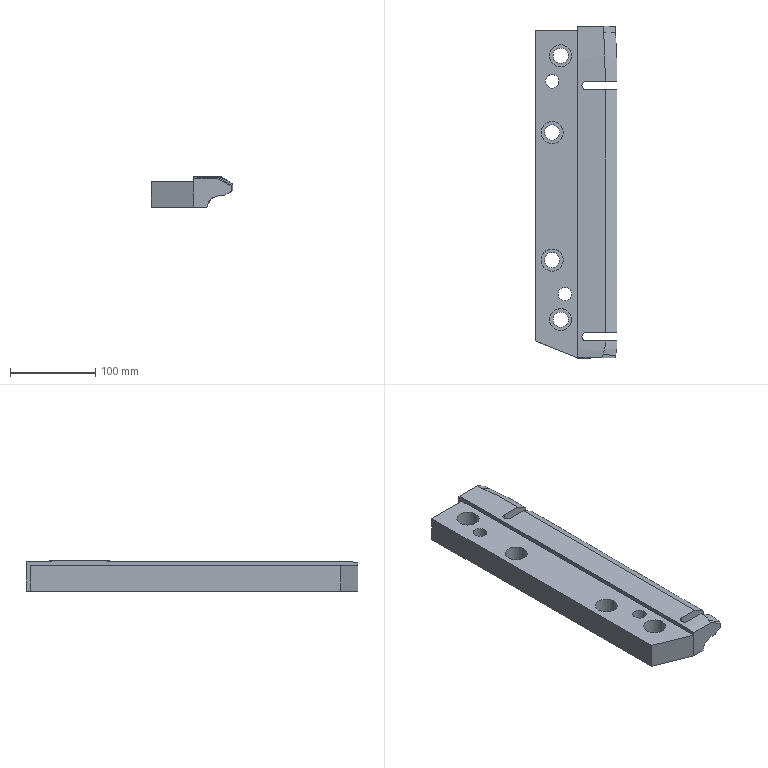Part | NX | features solid 2 | 1 solid | 60 faces | box 96.035 x 390.001 x 35.682 mm | volume 919192 mm3 | spline 32 | plane 16 | cylinder 12 | commonest cylinder face diameters 18 x4 26 x4 10 x2 16 x2